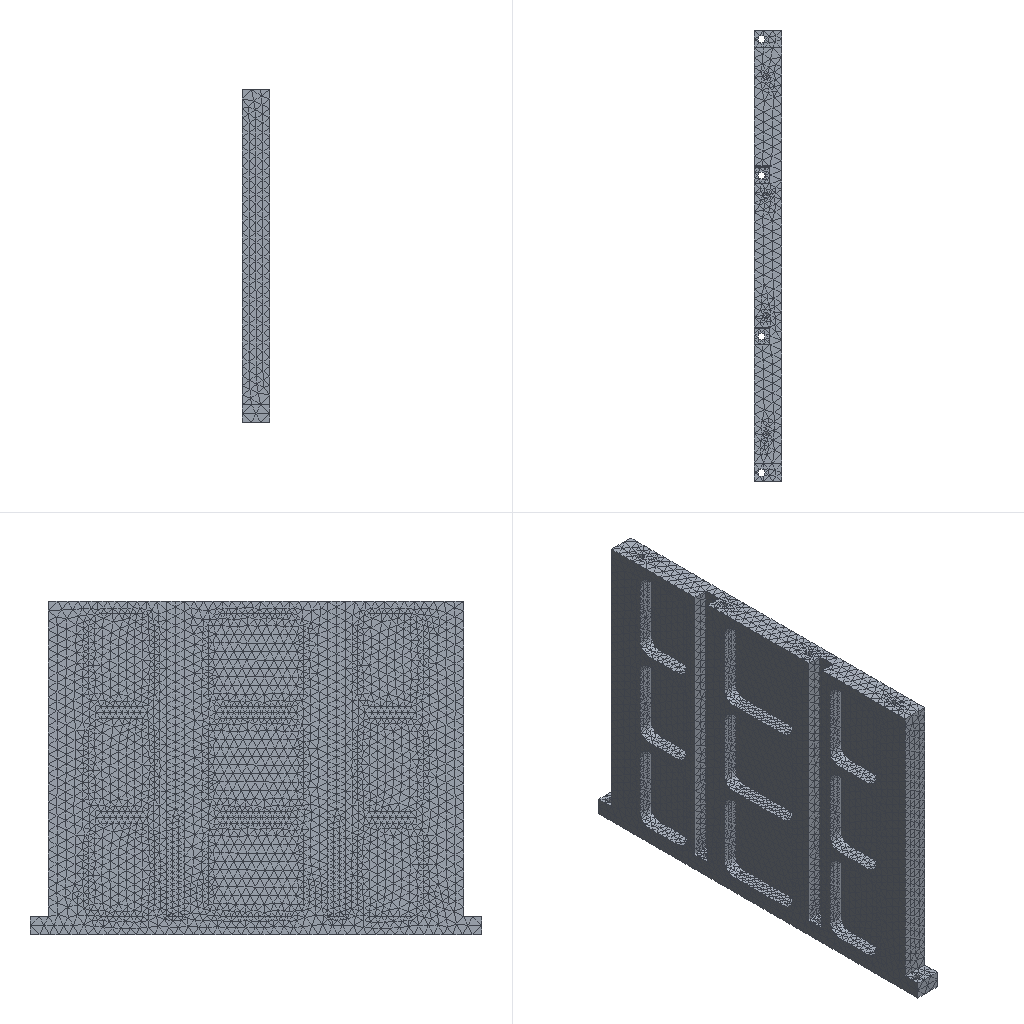Simulation study | nx simcenter
Set-up summary:
category,name,step,type,value,unit,region
solver,nx_nastran (Simcenter)
units,not stated in the deck,,not stated
analysis,deck,,static,static
analysis,solution,,SOL,101
load_step,SUBCASE 1,1,SUBCASE,SPC=1 LOAD=2
load_step,requested,,,1
mesh,nodes,,,50207
mesh,elements,,,27321
element_type,CTETRA,,solid,27321
load,nodal force total,,FX,0.0,model units
load,nodal force total,,FY,0.0,model units
load,nodal force total,,FZ,-2999999.894,model units
load,load commands in deck,,count,607
bc,support commands in deck,,count,949
analysis,NX solution 0,,Structural,Linear Statics - Single Constraint
check,setup vs results,,match,every grid point's frame and coordinates and every element id; grid points of CTETRA elements
Nastran input file, long lists of numbers shortened:
$*$$$$$$$$$$$$$$$$$$$$$$$$$$$$$$$$$$$$$$$$$$$$$$$$$$$$$$$$$$$$$$$$$
$*
$*                    NX v10.0.0.24 TRANSLATOR
$*                    FOR NX NASTRAN VERSION 10.0
$ (33 more lines like these left out)
ASSIGN OUTPUT2='108_sim1-solution_1.op2' UNIT=12
$*
$*$$$$$$$$$$$$$$$$$$$$$$$$$$$$$$$$$$$
$*
$* EXECUTIVE CONTROL
$*
$*$$$$$$$$$$$$$$$$$$$$$$$$$$$$$$$$$$$
$*
ID,NASTRAN,108_sim1-solution_1
SOL 101
CEND
$*
$*$$$$$$$$$$$$$$$$$$$$$$$$$$$$$$$$$$$
$*
$* CASE CONTROL
$*
$*$$$$$$$$$$$$$$$$$$$$$$$$$$$$$$$$$$$
$*
TITLE = Solution 1
ECHO = NONE
SPC = 1
OUTPUT
BCRESULTS(TRACTION,FORCE,PLOT) = ALL
DISPLACEMENT(PLOT) = ALL
ESE(PLOT) = ALL
FORCE(PLOT,CORNER) = ALL
OLOAD(PLOT) = ALL
SPCFORCES(PLOT) = ALL
STRAIN(PLOT,FIBER,CORNER) = ALL
STRESS(PLOT,CORNER) = ALL
$*  NX Step: Subcase - Static Loads 1
SUBCASE 1
LABEL = Subcase - Static Loads 1
LOAD = 2
$*
$*$$$$$$$$$$$$$$$$$$$$$$$$$$$$$$$$$$$
$*
$* BULK DATA
$*
$*$$$$$$$$$$$$$$$$$$$$$$$$$$$$$$$$$$$
$*
BEGIN BULK
$*
$* PARAM CARDS
$*
PARAM      K6ROT100.0000
PARAM     OIBULK     YES
PARAM    OMACHPR     YES
PARAM       POST      -2
PARAM    POSTEXT     YES
PARAM    UNITSYS   MN-MM
$*
$* GRID CARDS
$*
GRID*              50008               0-2.300000000E+01-1.890000000E+02+
*       1.5000000000E+01               0
GRID*              50009               0-2.300000000E+01-1.890000000E+02+
*       0.0000000000E+00               0
$ (100410 more lines like these left out)
$*
$* ELEMENT CARDS
$*
$*  NX Mesh Collector: Solid(1)
$*  NX Mesh: 3d_mesh(1)
CTETRA         1       1       1   38824   38816   38815    1220   43282+
+           1221    1222   43281   43250
CTETRA         2       1       1   38820       2   38815    1223    1224+
+           1225    1222   43249    1226
$ (54638 more lines like these left out)
$*
$* PROPERTY CARDS
$*
$*  NX Property: PSOLID1
PSOLID         1       1       0                           SMECH
$*
$* MATERIAL CARDS
$*
$*  NX Material: Aluminum_6061
MAT1           16.8980+7        0.3300002.7110-62.2161-5
MATT1          1       1               2               3
TABLEM1        1                                                        +
+        20.00006.8980+7 21.11006.8980+7 23.89006.8980+7 37.78006.8290+7+
+        51.67006.8290+7 65.56006.7600+7 79.44006.6910+7 93.33006.6221+7+
+       107.22006.5531+7121.11006.4841+7135.00006.4151+7148.89006.3461+7+
+       162.78006.2772+7176.67006.1392+7190.56006.0702+7204.44005.9323+7+
+       218.33005.8633+7232.22005.7253+7246.11005.5874+7260.00005.4494+7+
+       273.89005.3114+7287.78005.1735+7301.67005.0355+7315.56004.8976+7+
+       329.44004.7596+7343.33004.6216+7357.22004.4147+7371.11004.2767+7+
+       385.00004.1388+7398.89003.9318+7412.78003.7939+7426.67003.5869+7+
+           ENDT
TABLEM1        2                                                        +
+        20.00000.330000 21.11000.330000    ENDT
TABLEM1        3                                                        +
+        20.00002.2380-5 93.33002.3184-5107.22002.3346-5121.11002.3508-5+
+       135.00002.3670-5148.89002.3832-5162.78002.3994-5176.67002.4138-5+
+       190.56002.4300-5204.44002.4444-5218.33002.4588-5232.22002.4732-5+
+       246.11002.4876-5260.00002.5002-5273.89002.5146-5287.78002.5272-5+
+       301.67002.5398-5315.56002.5524-5    ENDT
$*
$* LOAD AND CONSTRAINT CARDS
$*
$*  NX Load and Constraint: Fixed(1)
SPC            1   44579  123456  0.0000
SPC            1   44580  123456  0.0000
SPC            1   44581  123456  0.0000
SPC            1   44582  123456  0.0000
$ (945 more lines like these left out)
$*  NX Load and Constraint: Force(1)
FORCE          2   45396       0 3094.47  0.0000  0.0000-1.00000
FORCE          2   45397       0 3494.46  0.0000  0.0000-1.00000
FORCE          2   45398       0 3751.96  0.0000  0.0000-1.00000
FORCE          2   45399       0 4025.70  0.0000  0.0000-1.00000
$ (603 more lines like these left out)
ENDDATA d22d5d4b
Results summary:
result,analysis,,,static
result,last_loadstep,,,1
result,primary field,,,displacements
result,max displacement,,,0.02323,model units
result,reaction total,,FX,0.0564,model units
result,reaction total,,FY,-0.01593,model units
result,reaction total,,FZ,3000002.0,model units
result,NX solution 0,,loadcases,1,mm